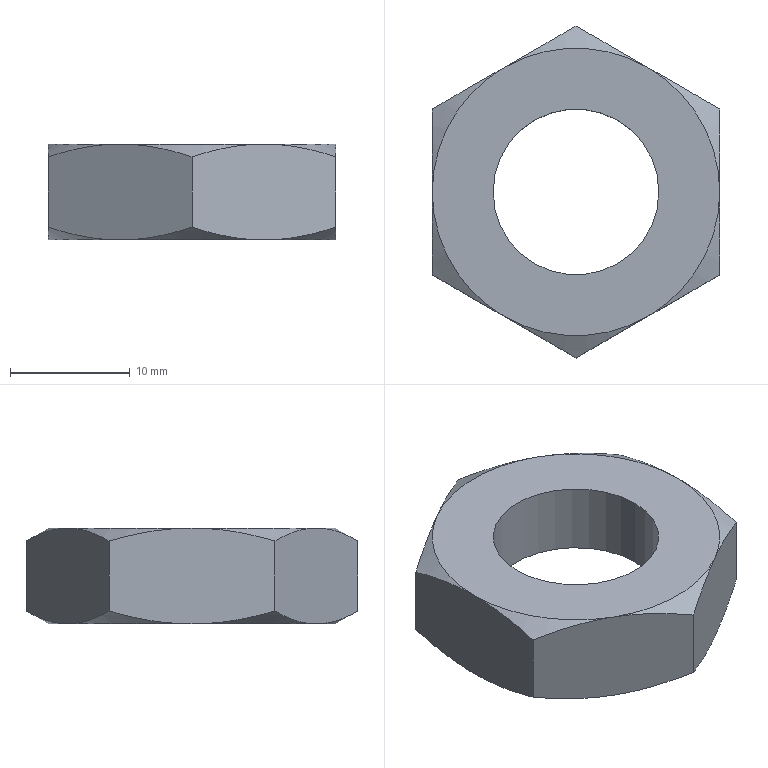Part | STEP file | HXGR200008-06-03-06_M16 | 1 solid | 25 faces | box 24 x 27.713 x 8 mm | volume 2461 mm3 | cone 12 | plane 9 | cylinder 4 | commonest cylinder face diameters 13.835 x2 19.5 x2
STEP:
#1=CARTESIAN_POINT('',(9.75,0.,2.));
#2=VERTEX_POINT('',#1);
#3=CARTESIAN_POINT('',(-9.75,0.,2.));
#4=VERTEX_POINT('',#3);
#5=CARTESIAN_POINT('',(0.,0.,2.));
#6=DIRECTION('',(0.,0.,-1.));
#7=DIRECTION('',(-1.,0.,0.));
#8=AXIS2_PLACEMENT_3D('',#5,#6,#7);
#9=CIRCLE('',#8,9.75);
#10=EDGE_CURVE('',#2,#4,#9,.T.);
#11=ORIENTED_EDGE('',*,*,#10,.F.);
#12=CARTESIAN_POINT('',(9.75,0.,0.));
#13=VERTEX_POINT('',#12);
#14=CARTESIAN_POINT('',(9.75,0.,2.));
#15=DIRECTION('',(0.,0.,-1.));
#16=VECTOR('',#15,1000.);
#17=LINE('',#14,#16);
#18=EDGE_CURVE('',#2,#13,#17,.T.);
#19=ORIENTED_EDGE('',*,*,#18,.T.);
#20=CARTESIAN_POINT('',(-9.75,0.,0.));
#21=VERTEX_POINT('',#20);
#22=CARTESIAN_POINT('',(0.,0.,0.));
#23=DIRECTION('',(0.,0.,-1.));
#24=DIRECTION('',(-1.,0.,0.));
#25=AXIS2_PLACEMENT_3D('',#22,#23,#24);
#26=CIRCLE('',#25,9.75);
#27=EDGE_CURVE('',#13,#21,#26,.T.);
#28=ORIENTED_EDGE('',*,*,#27,.T.);
#29=CARTESIAN_POINT('',(-9.75,0.,2.));
#30=DIRECTION('',(0.,0.,-1.));
#31=VECTOR('',#30,1000.);
#32=LINE('',#29,#31);
#33=EDGE_CURVE('',#4,#21,#32,.T.);
#34=ORIENTED_EDGE('',*,*,#33,.F.);
#35=EDGE_LOOP('',(#11,#19,#28,#34));
#36=FACE_OUTER_BOUND('',#35,.T.);
#37=CARTESIAN_POINT('',(0.,0.,2.));
#38=DIRECTION('',(0.,0.,-1.));
#39=DIRECTION('',(-1.,0.,0.));
#40=AXIS2_PLACEMENT_3D('',#37,#38,#39);
#41=CYLINDRICAL_SURFACE('',#40,9.75);
#42=ADVANCED_FACE('',(#36),#41,.F.);
#43=CARTESIAN_POINT('',(-6.918,0.,8.));
#44=VERTEX_POINT('',#43);
#45=CARTESIAN_POINT('',(6.918,0.,8.));
#46=VERTEX_POINT('',#45);
#47=CARTESIAN_POINT('',(0.,0.,8.));
#48=DIRECTION('',(0.,0.,1.));
#49=DIRECTION('',(1.,0.,0.));
#50=AXIS2_PLACEMENT_3D('',#47,#48,#49);
#51=CIRCLE('',#50,6.918);
#52=EDGE_CURVE('',#44,#46,#51,.T.);
#53=ORIENTED_EDGE('',*,*,#52,.T.);
#54=CARTESIAN_POINT('',(6.918,0.,2.));
#55=VERTEX_POINT('',#54);
#56=CARTESIAN_POINT('',(6.918,0.,8.));
#57=DIRECTION('',(0.,0.,-1.));
#58=VECTOR('',#57,1000.);
#59=LINE('',#56,#58);
#60=EDGE_CURVE('',#46,#55,#59,.T.);
#61=ORIENTED_EDGE('',*,*,#60,.T.);
#62=CARTESIAN_POINT('',(-6.918,0.,2.));
#63=VERTEX_POINT('',#62);
#64=CARTESIAN_POINT('',(0.,0.,2.));
#65=DIRECTION('',(0.,0.,-1.));
#66=DIRECTION('',(-1.,0.,0.));
#67=AXIS2_PLACEMENT_3D('',#64,#65,#66);
#68=CIRCLE('',#67,6.918);
#69=EDGE_CURVE('',#55,#63,#68,.T.);
#70=ORIENTED_EDGE('',*,*,#69,.T.);
#71=CARTESIAN_POINT('',(-6.918,0.,8.));
#72=DIRECTION('',(0.,0.,-1.));
#73=VECTOR('',#72,1000.);
#74=LINE('',#71,#73);
#75=EDGE_CURVE('',#44,#63,#74,.T.);
#76=ORIENTED_EDGE('',*,*,#75,.F.);
#77=EDGE_LOOP('',(#53,#61,#70,#76));
#78=FACE_OUTER_BOUND('',#77,.T.);
#79=CARTESIAN_POINT('',(0.,0.,8.));
#80=DIRECTION('',(0.,0.,-1.));
#81=DIRECTION('',(-1.,0.,0.));
#82=AXIS2_PLACEMENT_3D('',#79,#80,#81);
#83=CYLINDRICAL_SURFACE('',#82,6.918);
#84=ADVANCED_FACE('',(#78),#83,.F.);
#85=ORIENTED_EDGE('',*,*,#60,.F.);
#86=CARTESIAN_POINT('',(0.,0.,8.));
#87=DIRECTION('',(0.,0.,1.));
#88=DIRECTION('',(1.,0.,0.));
#89=AXIS2_PLACEMENT_3D('',#86,#87,#88);
#90=CIRCLE('',#89,6.918);
#91=EDGE_CURVE('',#46,#44,#90,.T.);
#92=ORIENTED_EDGE('',*,*,#91,.T.);
#93=ORIENTED_EDGE('',*,*,#75,.T.);
#94=CARTESIAN_POINT('',(0.,0.,2.));
#95=DIRECTION('',(0.,0.,-1.));
#96=DIRECTION('',(-1.,0.,0.));
#97=AXIS2_PLACEMENT_3D('',#94,#95,#96);
#98=CIRCLE('',#97,6.918);
#99=EDGE_CURVE('',#63,#55,#98,.T.);
#100=ORIENTED_EDGE('',*,*,#99,.T.);
#101=EDGE_LOOP('',(#85,#92,#93,#100));
#102=FACE_OUTER_BOUND('',#101,.T.);
#103=CARTESIAN_POINT('',(0.,0.,8.));
#104=DIRECTION('',(0.,0.,-1.));
#105=DIRECTION('',(-1.,0.,0.));
#106=AXIS2_PLACEMENT_3D('',#103,#104,#105);
#107=CYLINDRICAL_SURFACE('',#106,6.918);
#108=ADVANCED_FACE('',(#102),#107,.F.);
#109=CARTESIAN_POINT('',(12.,6.928,6.928));
#110=VERTEX_POINT('',#109);
#111=CARTESIAN_POINT('',(6.,10.392,8.));
#112=VERTEX_POINT('',#111);
#113=CARTESIAN_POINT('',(12.,6.928,6.928));
#114=CARTESIAN_POINT('',(11.018,7.495,7.255));
#115=CARTESIAN_POINT('',(10.03,8.066,7.525));
#116=CARTESIAN_POINT('',(8.032,9.219,7.898));
#117=CARTESIAN_POINT('',(7.022,9.802,8.));
#118=CARTESIAN_POINT('',(6.,10.392,8.));
#119=B_SPLINE_CURVE_WITH_KNOTS('',3,(#113,#114,#115,#116,#117,#118),.UNSPECIFIED.,.F.,.F.,(4,2,4),(0.000000238,0.003505,0.00701),.UNSPECIFIED.);
#120=EDGE_CURVE('',#110,#112,#119,.T.);
#121=ORIENTED_EDGE('',*,*,#120,.F.);
#122=CARTESIAN_POINT('',(12.,6.928,1.072));
#123=VERTEX_POINT('',#122);
#124=CARTESIAN_POINT('',(12.,6.928,8.));
#125=DIRECTION('',(0.,0.,-1.));
#126=VECTOR('',#125,1000.);
#127=LINE('',#124,#126);
#128=EDGE_CURVE('',#110,#123,#127,.T.);
#129=ORIENTED_EDGE('',*,*,#128,.T.);
#130=CARTESIAN_POINT('',(6.,10.392,0.));
#131=VERTEX_POINT('',#130);
#132=CARTESIAN_POINT('',(6.,10.392,0.));
#133=CARTESIAN_POINT('',(6.509,10.098,0.));
#134=CARTESIAN_POINT('',(7.021,9.803,0.02533));
#135=CARTESIAN_POINT('',(8.033,9.219,0.1234));
#136=CARTESIAN_POINT('',(8.535,8.929,0.196));
#137=CARTESIAN_POINT('',(10.034,8.063,0.476));
#138=CARTESIAN_POINT('',(11.021,7.493,0.7454));
#139=CARTESIAN_POINT('',(12.,6.928,1.072));
#140=B_SPLINE_CURVE_WITH_KNOTS('',3,(#132,#133,#134,#135,#136,#137,#138,#139),.UNSPECIFIED.,.F.,.F.,(4,2,2,4),(0.00701,0.008756,0.0105,0.01399),.UNSPECIFIED.);
#141=EDGE_CURVE('',#131,#123,#140,.T.);
#142=ORIENTED_EDGE('',*,*,#141,.F.);
#143=CARTESIAN_POINT('',(0.,13.856,1.072));
#144=VERTEX_POINT('',#143);
#145=CARTESIAN_POINT('',(0.,13.856,1.072));
#146=CARTESIAN_POINT('',(0.9815,13.29,0.7446));
#147=CARTESIAN_POINT('',(1.97,12.719,0.4751));
#148=CARTESIAN_POINT('',(3.968,11.565,0.1021));
#149=CARTESIAN_POINT('',(4.978,10.982,0.));
#150=CARTESIAN_POINT('',(6.,10.392,0.));
#151=B_SPLINE_CURVE_WITH_KNOTS('',3,(#145,#146,#147,#148,#149,#150),.UNSPECIFIED.,.F.,.F.,(4,2,4),(0.000000238,0.003505,0.00701),.UNSPECIFIED.);
#152=EDGE_CURVE('',#144,#131,#151,.T.);
#153=ORIENTED_EDGE('',*,*,#152,.F.);
#154=CARTESIAN_POINT('',(0.,13.856,6.928));
#155=VERTEX_POINT('',#154);
#156=CARTESIAN_POINT('',(0.,13.856,8.));
#157=DIRECTION('',(0.,0.,-1.));
#158=VECTOR('',#157,1000.);
#159=LINE('',#156,#158);
#160=EDGE_CURVE('',#155,#144,#159,.T.);
#161=ORIENTED_EDGE('',*,*,#160,.F.);
#162=CARTESIAN_POINT('',(6.,10.392,8.));
#163=CARTESIAN_POINT('',(5.491,10.686,8.));
#164=CARTESIAN_POINT('',(4.979,10.982,7.975));
#165=CARTESIAN_POINT('',(3.967,11.566,7.877));
#166=CARTESIAN_POINT('',(3.465,11.856,7.804));
#167=CARTESIAN_POINT('',(1.966,12.721,7.524));
#168=CARTESIAN_POINT('',(0.9791,13.291,7.255));
#169=CARTESIAN_POINT('',(0.,13.856,6.928));
#170=B_SPLINE_CURVE_WITH_KNOTS('',3,(#162,#163,#164,#165,#166,#167,#168,#169),.UNSPECIFIED.,.F.,.F.,(4,2,2,4),(0.00701,0.008756,0.0105,0.01399),.UNSPECIFIED.);
#171=EDGE_CURVE('',#112,#155,#170,.T.);
#172=ORIENTED_EDGE('',*,*,#171,.F.);
#173=EDGE_LOOP('',(#121,#129,#142,#153,#161,#172));
#174=FACE_OUTER_BOUND('',#173,.T.);
#175=CARTESIAN_POINT('',(12.,6.928,8.));
#176=DIRECTION('',(-0.5,-0.866,0.));
#177=DIRECTION('',(0.866,-0.5,0.));
#178=AXIS2_PLACEMENT_3D('',#175,#176,#177);
#179=PLANE('',#178);
#180=ADVANCED_FACE('',(#174),#179,.F.);
#181=CARTESIAN_POINT('',(-6.,10.392,8.));
#182=VERTEX_POINT('',#181);
#183=CARTESIAN_POINT('',(0.,13.856,6.928));
#184=CARTESIAN_POINT('',(-0.9815,13.29,7.255));
#185=CARTESIAN_POINT('',(-1.97,12.719,7.525));
#186=CARTESIAN_POINT('',(-3.968,11.565,7.898));
#187=CARTESIAN_POINT('',(-4.978,10.982,8.));
#188=CARTESIAN_POINT('',(-6.,10.392,8.));
#189=B_SPLINE_CURVE_WITH_KNOTS('',3,(#183,#184,#185,#186,#187,#188),.UNSPECIFIED.,.F.,.F.,(4,2,4),(0.000000238,0.003505,0.00701),.UNSPECIFIED.);
#190=EDGE_CURVE('',#155,#182,#189,.T.);
#191=ORIENTED_EDGE('',*,*,#190,.F.);
#192=ORIENTED_EDGE('',*,*,#160,.T.);
#193=CARTESIAN_POINT('',(-6.,10.392,0.));
#194=VERTEX_POINT('',#193);
#195=CARTESIAN_POINT('',(-6.,10.392,0.));
#196=CARTESIAN_POINT('',(-5.491,10.686,0.));
#197=CARTESIAN_POINT('',(-4.979,10.982,0.02533));
#198=CARTESIAN_POINT('',(-3.967,11.566,0.1234));
#199=CARTESIAN_POINT('',(-3.465,11.856,0.196));
#200=CARTESIAN_POINT('',(-1.966,12.721,0.476));
#201=CARTESIAN_POINT('',(-0.9791,13.291,0.7454));
#202=CARTESIAN_POINT('',(0.,13.856,1.072));
#203=B_SPLINE_CURVE_WITH_KNOTS('',3,(#195,#196,#197,#198,#199,#200,#201,#202),.UNSPECIFIED.,.F.,.F.,(4,2,2,4),(0.00701,0.008756,0.0105,0.01399),.UNSPECIFIED.);
#204=EDGE_CURVE('',#194,#144,#203,.T.);
#205=ORIENTED_EDGE('',*,*,#204,.F.);
#206=CARTESIAN_POINT('',(-12.,6.928,1.072));
#207=VERTEX_POINT('',#206);
#208=CARTESIAN_POINT('',(-12.,6.928,1.072));
#209=CARTESIAN_POINT('',(-11.018,7.495,0.7446));
#210=CARTESIAN_POINT('',(-10.03,8.066,0.4751));
#211=CARTESIAN_POINT('',(-8.032,9.219,0.1021));
#212=CARTESIAN_POINT('',(-7.022,9.802,0.));
#213=CARTESIAN_POINT('',(-6.,10.392,0.));
#214=B_SPLINE_CURVE_WITH_KNOTS('',3,(#208,#209,#210,#211,#212,#213),.UNSPECIFIED.,.F.,.F.,(4,2,4),(0.000000238,0.003505,0.00701),.UNSPECIFIED.);
#215=EDGE_CURVE('',#207,#194,#214,.T.);
#216=ORIENTED_EDGE('',*,*,#215,.F.);
#217=CARTESIAN_POINT('',(-12.,6.928,6.928));
#218=VERTEX_POINT('',#217);
#219=CARTESIAN_POINT('',(-12.,6.928,8.));
#220=DIRECTION('',(0.,0.,-1.));
#221=VECTOR('',#220,1000.);
#222=LINE('',#219,#221);
#223=EDGE_CURVE('',#218,#207,#222,.T.);
#224=ORIENTED_EDGE('',*,*,#223,.F.);
#225=CARTESIAN_POINT('',(-6.,10.392,8.));
#226=CARTESIAN_POINT('',(-6.509,10.098,8.));
#227=CARTESIAN_POINT('',(-7.021,9.803,7.975));
#228=CARTESIAN_POINT('',(-8.033,9.219,7.877));
#229=CARTESIAN_POINT('',(-8.535,8.929,7.804));
#230=CARTESIAN_POINT('',(-10.034,8.063,7.524));
#231=CARTESIAN_POINT('',(-11.021,7.493,7.255));
#232=CARTESIAN_POINT('',(-12.,6.928,6.928));
#233=B_SPLINE_CURVE_WITH_KNOTS('',3,(#225,#226,#227,#228,#229,#230,#231,#232),.UNSPECIFIED.,.F.,.F.,(4,2,2,4),(0.00701,0.008756,0.0105,0.01399),.UNSPECIFIED.);
#234=EDGE_CURVE('',#182,#218,#233,.T.);
#235=ORIENTED_EDGE('',*,*,#234,.F.);
#236=EDGE_LOOP('',(#191,#192,#205,#216,#224,#235));
#237=FACE_OUTER_BOUND('',#236,.T.);
#238=CARTESIAN_POINT('',(0.,13.856,8.));
#239=DIRECTION('',(0.5,-0.866,0.));
#240=DIRECTION('',(0.866,0.5,0.));
#241=AXIS2_PLACEMENT_3D('',#238,#239,#240);
#242=PLANE('',#241);
#243=ADVANCED_FACE('',(#237),#242,.F.);
#244=CARTESIAN_POINT('',(-12.,0.,8.));
#245=VERTEX_POINT('',#244);
#246=CARTESIAN_POINT('',(-12.,6.928,6.928));
#247=CARTESIAN_POINT('',(-12.,5.808,7.252));
#248=CARTESIAN_POINT('',(-12.,4.673,7.521));
#249=CARTESIAN_POINT('',(-12.,2.939,7.802));
#250=CARTESIAN_POINT('',(-12.,2.355,7.876));
#251=CARTESIAN_POINT('',(-12.,1.176,7.975));
#252=CARTESIAN_POINT('',(-12.,0.5865,8.));
#253=CARTESIAN_POINT('',(-12.,0.,8.));
#254=B_SPLINE_CURVE_WITH_KNOTS('',3,(#246,#247,#248,#249,#250,#251,#252,#253),.UNSPECIFIED.,.F.,.F.,(4,2,2,4),(0.03616,0.03967,0.04143,0.04318),.UNSPECIFIED.);
#255=EDGE_CURVE('',#218,#245,#254,.T.);
#256=ORIENTED_EDGE('',*,*,#255,.F.);
#257=ORIENTED_EDGE('',*,*,#223,.T.);
#258=CARTESIAN_POINT('',(-12.,0.,0.));
#259=VERTEX_POINT('',#258);
#260=CARTESIAN_POINT('',(-12.,0.,0.));
#261=CARTESIAN_POINT('',(-12.,0.5865,0.));
#262=CARTESIAN_POINT('',(-12.,1.176,0.02506));
#263=CARTESIAN_POINT('',(-12.,2.355,0.1242));
#264=CARTESIAN_POINT('',(-12.,2.939,0.1976));
#265=CARTESIAN_POINT('',(-12.,4.673,0.4791));
#266=CARTESIAN_POINT('',(-12.,5.808,0.7483));
#267=CARTESIAN_POINT('',(-12.,6.928,1.072));
#268=B_SPLINE_CURVE_WITH_KNOTS('',3,(#260,#261,#262,#263,#264,#265,#266,#267),.UNSPECIFIED.,.F.,.F.,(4,2,2,4),(0.01983,0.02158,0.02334,0.02685),.UNSPECIFIED.);
#269=EDGE_CURVE('',#259,#207,#268,.T.);
#270=ORIENTED_EDGE('',*,*,#269,.F.);
#271=CARTESIAN_POINT('',(-12.,-6.928,1.072));
#272=VERTEX_POINT('',#271);
#273=CARTESIAN_POINT('',(-12.,-6.928,1.072));
#274=CARTESIAN_POINT('',(-12.,-5.8,0.7461));
#275=CARTESIAN_POINT('',(-12.,-4.647,0.4736));
#276=CARTESIAN_POINT('',(-12.,-2.335,0.1008));
#277=CARTESIAN_POINT('',(-12.,-1.172,0.));
#278=CARTESIAN_POINT('',(-12.,0.,0.));
#279=B_SPLINE_CURVE_WITH_KNOTS('',3,(#273,#274,#275,#276,#277,#278),.UNSPECIFIED.,.F.,.F.,(4,2,4),(0.01282,0.01632,0.01983),.UNSPECIFIED.);
#280=EDGE_CURVE('',#272,#259,#279,.T.);
#281=ORIENTED_EDGE('',*,*,#280,.F.);
#282=CARTESIAN_POINT('',(-12.,-6.928,6.928));
#283=VERTEX_POINT('',#282);
#284=CARTESIAN_POINT('',(-12.,-6.928,8.));
#285=DIRECTION('',(0.,0.,-1.));
#286=VECTOR('',#285,1000.);
#287=LINE('',#284,#286);
#288=EDGE_CURVE('',#283,#272,#287,.T.);
#289=ORIENTED_EDGE('',*,*,#288,.F.);
#290=CARTESIAN_POINT('',(-12.,0.,8.));
#291=CARTESIAN_POINT('',(-12.,-1.172,8.));
#292=CARTESIAN_POINT('',(-12.,-2.335,7.899));
#293=CARTESIAN_POINT('',(-12.,-4.647,7.526));
#294=CARTESIAN_POINT('',(-12.,-5.8,7.254));
#295=CARTESIAN_POINT('',(-12.,-6.928,6.928));
#296=B_SPLINE_CURVE_WITH_KNOTS('',3,(#290,#291,#292,#293,#294,#295),.UNSPECIFIED.,.F.,.F.,(4,2,4),(0.04318,0.04669,0.05019),.UNSPECIFIED.);
#297=EDGE_CURVE('',#245,#283,#296,.T.);
#298=ORIENTED_EDGE('',*,*,#297,.F.);
#299=EDGE_LOOP('',(#256,#257,#270,#281,#289,#298));
#300=FACE_OUTER_BOUND('',#299,.T.);
#301=CARTESIAN_POINT('',(-12.,6.928,8.));
#302=DIRECTION('',(1.,0.,0.));
#303=DIRECTION('',(0.,1.,0.));
#304=AXIS2_PLACEMENT_3D('',#301,#302,#303);
#305=PLANE('',#304);
#306=ADVANCED_FACE('',(#300),#305,.F.);
#307=CARTESIAN_POINT('',(-6.,-10.392,8.));
#308=VERTEX_POINT('',#307);
#309=CARTESIAN_POINT('',(-12.,-6.928,6.928));
#310=CARTESIAN_POINT('',(-11.018,-7.495,7.255));
#311=CARTESIAN_POINT('',(-10.03,-8.066,7.525));
#312=CARTESIAN_POINT('',(-8.032,-9.219,7.898));
#313=CARTESIAN_POINT('',(-7.022,-9.802,8.));
#314=CARTESIAN_POINT('',(-6.,-10.392,8.));
#315=B_SPLINE_CURVE_WITH_KNOTS('',3,(#309,#310,#311,#312,#313,#314),.UNSPECIFIED.,.F.,.F.,(4,2,4),(0.000000238,0.003505,0.00701),.UNSPECIFIED.);
#316=EDGE_CURVE('',#283,#308,#315,.T.);
#317=ORIENTED_EDGE('',*,*,#316,.F.);
#318=ORIENTED_EDGE('',*,*,#288,.T.);
#319=CARTESIAN_POINT('',(-6.,-10.392,0.));
#320=VERTEX_POINT('',#319);
#321=CARTESIAN_POINT('',(-6.,-10.392,0.));
#322=CARTESIAN_POINT('',(-6.509,-10.098,0.));
#323=CARTESIAN_POINT('',(-7.021,-9.803,0.02533));
#324=CARTESIAN_POINT('',(-8.033,-9.219,0.1234));
#325=CARTESIAN_POINT('',(-8.535,-8.929,0.196));
#326=CARTESIAN_POINT('',(-10.034,-8.063,0.476));
#327=CARTESIAN_POINT('',(-11.021,-7.493,0.7454));
#328=CARTESIAN_POINT('',(-12.,-6.928,1.072));
#329=B_SPLINE_CURVE_WITH_KNOTS('',3,(#321,#322,#323,#324,#325,#326,#327,#328),.UNSPECIFIED.,.F.,.F.,(4,2,2,4),(0.00701,0.008756,0.0105,0.01399),.UNSPECIFIED.);
#330=EDGE_CURVE('',#320,#272,#329,.T.);
#331=ORIENTED_EDGE('',*,*,#330,.F.);
#332=CARTESIAN_POINT('',(0.,-13.856,1.072));
#333=VERTEX_POINT('',#332);
#334=CARTESIAN_POINT('',(0.,-13.856,1.072));
#335=CARTESIAN_POINT('',(-0.9815,-13.29,0.7446));
#336=CARTESIAN_POINT('',(-1.97,-12.719,0.4751));
#337=CARTESIAN_POINT('',(-3.968,-11.565,0.1021));
#338=CARTESIAN_POINT('',(-4.978,-10.982,0.));
#339=CARTESIAN_POINT('',(-6.,-10.392,0.));
#340=B_SPLINE_CURVE_WITH_KNOTS('',3,(#334,#335,#336,#337,#338,#339),.UNSPECIFIED.,.F.,.F.,(4,2,4),(0.000000238,0.003505,0.00701),.UNSPECIFIED.);
#341=EDGE_CURVE('',#333,#320,#340,.T.);
#342=ORIENTED_EDGE('',*,*,#341,.F.);
#343=CARTESIAN_POINT('',(0.,-13.856,6.928));
#344=VERTEX_POINT('',#343);
#345=CARTESIAN_POINT('',(0.,-13.856,8.));
#346=DIRECTION('',(0.,0.,-1.));
#347=VECTOR('',#346,1000.);
#348=LINE('',#345,#347);
#349=EDGE_CURVE('',#344,#333,#348,.T.);
#350=ORIENTED_EDGE('',*,*,#349,.F.);
#351=CARTESIAN_POINT('',(-6.,-10.392,8.));
#352=CARTESIAN_POINT('',(-5.491,-10.686,8.));
#353=CARTESIAN_POINT('',(-4.979,-10.982,7.975));
#354=CARTESIAN_POINT('',(-3.967,-11.566,7.877));
#355=CARTESIAN_POINT('',(-3.465,-11.856,7.804));
#356=CARTESIAN_POINT('',(-1.966,-12.721,7.524));
#357=CARTESIAN_POINT('',(-0.9791,-13.291,7.255));
#358=CARTESIAN_POINT('',(0.,-13.856,6.928));
#359=B_SPLINE_CURVE_WITH_KNOTS('',3,(#351,#352,#353,#354,#355,#356,#357,#358),.UNSPECIFIED.,.F.,.F.,(4,2,2,4),(0.00701,0.008756,0.0105,0.01399),.UNSPECIFIED.);
#360=EDGE_CURVE('',#308,#344,#359,.T.);
#361=ORIENTED_EDGE('',*,*,#360,.F.);
#362=EDGE_LOOP('',(#317,#318,#331,#342,#350,#361));
#363=FACE_OUTER_BOUND('',#362,.T.);
#364=CARTESIAN_POINT('',(-12.,-6.928,8.));
#365=DIRECTION('',(0.5,0.866,0.));
#366=DIRECTION('',(-0.866,0.5,0.));
#367=AXIS2_PLACEMENT_3D('',#364,#365,#366);
#368=PLANE('',#367);
#369=ADVANCED_FACE('',(#363),#368,.F.);
#370=CARTESIAN_POINT('',(6.,-10.392,8.));
#371=VERTEX_POINT('',#370);
#372=CARTESIAN_POINT('',(0.,-13.856,6.928));
#373=CARTESIAN_POINT('',(0.9815,-13.29,7.255));
#374=CARTESIAN_POINT('',(1.97,-12.719,7.525));
#375=CARTESIAN_POINT('',(3.968,-11.565,7.898));
#376=CARTESIAN_POINT('',(4.978,-10.982,8.));
#377=CARTESIAN_POINT('',(6.,-10.392,8.));
#378=B_SPLINE_CURVE_WITH_KNOTS('',3,(#372,#373,#374,#375,#376,#377),.UNSPECIFIED.,.F.,.F.,(4,2,4),(0.000000238,0.003505,0.00701),.UNSPECIFIED.);
#379=EDGE_CURVE('',#344,#371,#378,.T.);
#380=ORIENTED_EDGE('',*,*,#379,.F.);
#381=ORIENTED_EDGE('',*,*,#349,.T.);
#382=CARTESIAN_POINT('',(6.,-10.392,0.));
#383=VERTEX_POINT('',#382);
#384=CARTESIAN_POINT('',(6.,-10.392,0.));
#385=CARTESIAN_POINT('',(5.491,-10.686,0.));
#386=CARTESIAN_POINT('',(4.979,-10.982,0.02533));
#387=CARTESIAN_POINT('',(3.967,-11.566,0.1234));
#388=CARTESIAN_POINT('',(3.465,-11.856,0.196));
#389=CARTESIAN_POINT('',(1.966,-12.721,0.476));
#390=CARTESIAN_POINT('',(0.9791,-13.291,0.7454));
#391=CARTESIAN_POINT('',(0.,-13.856,1.072));
#392=B_SPLINE_CURVE_WITH_KNOTS('',3,(#384,#385,#386,#387,#388,#389,#390,#391),.UNSPECIFIED.,.F.,.F.,(4,2,2,4),(0.00701,0.008756,0.0105,0.01399),.UNSPECIFIED.);
#393=EDGE_CURVE('',#383,#333,#392,.T.);
#394=ORIENTED_EDGE('',*,*,#393,.F.);
#395=CARTESIAN_POINT('',(12.,-6.928,1.072));
#396=VERTEX_POINT('',#395);
#397=CARTESIAN_POINT('',(12.,-6.928,1.072));
#398=CARTESIAN_POINT('',(11.018,-7.495,0.7446));
#399=CARTESIAN_POINT('',(10.03,-8.066,0.4751));
#400=CARTESIAN_POINT('',(8.032,-9.219,0.1021));
#401=CARTESIAN_POINT('',(7.022,-9.802,0.));
#402=CARTESIAN_POINT('',(6.,-10.392,0.));
#403=B_SPLINE_CURVE_WITH_KNOTS('',3,(#397,#398,#399,#400,#401,#402),.UNSPECIFIED.,.F.,.F.,(4,2,4),(0.000000238,0.003505,0.00701),.UNSPECIFIED.);
#404=EDGE_CURVE('',#396,#383,#403,.T.);
#405=ORIENTED_EDGE('',*,*,#404,.F.);
#406=CARTESIAN_POINT('',(12.,-6.928,6.928));
#407=VERTEX_POINT('',#406);
#408=CARTESIAN_POINT('',(12.,-6.928,8.));
#409=DIRECTION('',(0.,0.,-1.));
#410=VECTOR('',#409,1000.);
#411=LINE('',#408,#410);
#412=EDGE_CURVE('',#407,#396,#411,.T.);
#413=ORIENTED_EDGE('',*,*,#412,.F.);
#414=CARTESIAN_POINT('',(6.,-10.392,8.));
#415=CARTESIAN_POINT('',(6.509,-10.098,8.));
#416=CARTESIAN_POINT('',(7.021,-9.803,7.975));
#417=CARTESIAN_POINT('',(8.033,-9.219,7.877));
#418=CARTESIAN_POINT('',(8.535,-8.929,7.804));
#419=CARTESIAN_POINT('',(10.034,-8.063,7.524));
#420=CARTESIAN_POINT('',(11.021,-7.493,7.255));
#421=CARTESIAN_POINT('',(12.,-6.928,6.928));
#422=B_SPLINE_CURVE_WITH_KNOTS('',3,(#414,#415,#416,#417,#418,#419,#420,#421),.UNSPECIFIED.,.F.,.F.,(4,2,2,4),(0.00701,0.008756,0.0105,0.01399),.UNSPECIFIED.);
#423=EDGE_CURVE('',#371,#407,#422,.T.);
#424=ORIENTED_EDGE('',*,*,#423,.F.);
#425=EDGE_LOOP('',(#380,#381,#394,#405,#413,#424));
#426=FACE_OUTER_BOUND('',#425,.T.);
#427=CARTESIAN_POINT('',(0.,-13.856,8.));
#428=DIRECTION('',(-0.5,0.866,0.));
#429=DIRECTION('',(-0.866,-0.5,0.));
#430=AXIS2_PLACEMENT_3D('',#427,#428,#429);
#431=PLANE('',#430);
#432=ADVANCED_FACE('',(#426),#431,.F.);
#433=CARTESIAN_POINT('',(12.,0.,8.));
#434=VERTEX_POINT('',#433);
#435=CARTESIAN_POINT('',(12.,-6.928,6.928));
#436=CARTESIAN_POINT('',(12.,-5.8,7.254));
#437=CARTESIAN_POINT('',(12.,-4.647,7.526));
#438=CARTESIAN_POINT('',(12.,-2.335,7.899));
#439=CARTESIAN_POINT('',(12.,-1.172,8.));
#440=CARTESIAN_POINT('',(12.,0.,8.));
#441=B_SPLINE_CURVE_WITH_KNOTS('',3,(#435,#436,#437,#438,#439,#440),.UNSPECIFIED.,.F.,.F.,(4,2,4),(0.01282,0.01632,0.01983),.UNSPECIFIED.);
#442=EDGE_CURVE('',#407,#434,#441,.T.);
#443=ORIENTED_EDGE('',*,*,#442,.F.);
#444=ORIENTED_EDGE('',*,*,#412,.T.);
#445=CARTESIAN_POINT('',(12.,0.,0.));
#446=VERTEX_POINT('',#445);
#447=CARTESIAN_POINT('',(12.,0.,0.));
#448=CARTESIAN_POINT('',(12.,-1.172,0.));
#449=CARTESIAN_POINT('',(12.,-2.335,0.1008));
#450=CARTESIAN_POINT('',(12.,-4.647,0.4736));
#451=CARTESIAN_POINT('',(12.,-5.8,0.7461));
#452=CARTESIAN_POINT('',(12.,-6.928,1.072));
#453=B_SPLINE_CURVE_WITH_KNOTS('',3,(#447,#448,#449,#450,#451,#452),.UNSPECIFIED.,.F.,.F.,(4,2,4),(0.04318,0.04669,0.05019),.UNSPECIFIED.);
#454=EDGE_CURVE('',#446,#396,#453,.T.);
#455=ORIENTED_EDGE('',*,*,#454,.F.);
#456=CARTESIAN_POINT('',(12.,6.928,1.072));
#457=CARTESIAN_POINT('',(12.,5.808,0.7483));
#458=CARTESIAN_POINT('',(12.,4.673,0.4791));
#459=CARTESIAN_POINT('',(12.,2.939,0.1976));
#460=CARTESIAN_POINT('',(12.,2.355,0.1242));
#461=CARTESIAN_POINT('',(12.,1.176,0.02506));
#462=CARTESIAN_POINT('',(12.,0.5865,0.));
#463=CARTESIAN_POINT('',(12.,0.,0.));
#464=B_SPLINE_CURVE_WITH_KNOTS('',3,(#456,#457,#458,#459,#460,#461,#462,#463),.UNSPECIFIED.,.F.,.F.,(4,2,2,4),(0.03616,0.03967,0.04143,0.04318),.UNSPECIFIED.);
#465=EDGE_CURVE('',#123,#446,#464,.T.);
#466=ORIENTED_EDGE('',*,*,#465,.F.);
#467=ORIENTED_EDGE('',*,*,#128,.F.);
#468=CARTESIAN_POINT('',(12.,0.,8.));
#469=CARTESIAN_POINT('',(12.,0.5865,8.));
#470=CARTESIAN_POINT('',(12.,1.176,7.975));
#471=CARTESIAN_POINT('',(12.,2.355,7.876));
#472=CARTESIAN_POINT('',(12.,2.939,7.802));
#473=CARTESIAN_POINT('',(12.,4.673,7.521));
#474=CARTESIAN_POINT('',(12.,5.808,7.252));
#475=CARTESIAN_POINT('',(12.,6.928,6.928));
#476=B_SPLINE_CURVE_WITH_KNOTS('',3,(#468,#469,#470,#471,#472,#473,#474,#475),.UNSPECIFIED.,.F.,.F.,(4,2,2,4),(0.01983,0.02158,0.02334,0.02685),.UNSPECIFIED.);
#477=EDGE_CURVE('',#434,#110,#476,.T.);
#478=ORIENTED_EDGE('',*,*,#477,.F.);
#479=EDGE_LOOP('',(#443,#444,#455,#466,#467,#478));
#480=FACE_OUTER_BOUND('',#479,.T.);
#481=CARTESIAN_POINT('',(12.,-6.928,8.));
#482=DIRECTION('',(-1.,0.,0.));
#483=DIRECTION('',(0.,-1.,0.));
#484=AXIS2_PLACEMENT_3D('',#481,#482,#483);
#485=PLANE('',#484);
#486=ADVANCED_FACE('',(#480),#485,.F.);
#487=ORIENTED_EDGE('',*,*,#52,.F.);
#488=ORIENTED_EDGE('',*,*,#91,.F.);
#489=EDGE_LOOP('',(#487,#488));
#490=FACE_BOUND('',#489,.T.);
#491=CARTESIAN_POINT('',(0.,0.,8.));
#492=DIRECTION('',(0.,0.,-1.));
#493=DIRECTION('',(-1.,0.,0.));
#494=AXIS2_PLACEMENT_3D('',#491,#492,#493);
#495=CIRCLE('',#494,12.);
#496=EDGE_CURVE('',#245,#182,#495,.T.);
#497=ORIENTED_EDGE('',*,*,#496,.F.);
#498=CARTESIAN_POINT('',(0.,0.,8.));
#499=DIRECTION('',(0.,0.,-1.));
#500=DIRECTION('',(-1.,0.,0.));
#501=AXIS2_PLACEMENT_3D('',#498,#499,#500);
#502=CIRCLE('',#501,12.);
#503=EDGE_CURVE('',#308,#245,#502,.T.);
#504=ORIENTED_EDGE('',*,*,#503,.F.);
#505=CARTESIAN_POINT('',(0.,0.,8.));
#506=DIRECTION('',(0.,0.,-1.));
#507=DIRECTION('',(-1.,0.,0.));
#508=AXIS2_PLACEMENT_3D('',#505,#506,#507);
#509=CIRCLE('',#508,12.);
#510=EDGE_CURVE('',#371,#308,#509,.T.);
#511=ORIENTED_EDGE('',*,*,#510,.F.);
#512=CARTESIAN_POINT('',(0.,0.,8.));
#513=DIRECTION('',(0.,0.,-1.));
#514=DIRECTION('',(-1.,0.,0.));
#515=AXIS2_PLACEMENT_3D('',#512,#513,#514);
#516=CIRCLE('',#515,12.);
#517=EDGE_CURVE('',#434,#371,#516,.T.);
#518=ORIENTED_EDGE('',*,*,#517,.F.);
#519=CARTESIAN_POINT('',(0.,0.,8.));
#520=DIRECTION('',(0.,0.,1.));
#521=DIRECTION('',(1.,0.,0.));
#522=AXIS2_PLACEMENT_3D('',#519,#520,#521);
#523=CIRCLE('',#522,12.);
#524=EDGE_CURVE('',#434,#112,#523,.T.);
#525=ORIENTED_EDGE('',*,*,#524,.T.);
#526=CARTESIAN_POINT('',(0.,0.,8.));
#527=DIRECTION('',(0.,0.,-1.));
#528=DIRECTION('',(-1.,0.,0.));
#529=AXIS2_PLACEMENT_3D('',#526,#527,#528);
#530=CIRCLE('',#529,12.);
#531=EDGE_CURVE('',#182,#112,#530,.T.);
#532=ORIENTED_EDGE('',*,*,#531,.F.);
#533=EDGE_LOOP('',(#497,#504,#511,#518,#525,#532));
#534=FACE_OUTER_BOUND('',#533,.T.);
#535=CARTESIAN_POINT('',(12.,6.928,8.));
#536=DIRECTION('',(0.,0.,-1.));
#537=DIRECTION('',(-1.,0.,0.));
#538=AXIS2_PLACEMENT_3D('',#535,#536,#537);
#539=PLANE('',#538);
#540=ADVANCED_FACE('',(#490,#534),#539,.F.);
#541=CARTESIAN_POINT('',(0.,0.,0.));
#542=DIRECTION('',(0.,0.,-1.));
#543=DIRECTION('',(-1.,0.,0.));
#544=AXIS2_PLACEMENT_3D('',#541,#542,#543);
#545=CIRCLE('',#544,9.75);
#546=EDGE_CURVE('',#21,#13,#545,.T.);
#547=ORIENTED_EDGE('',*,*,#546,.F.);
#548=ORIENTED_EDGE('',*,*,#27,.F.);
#549=EDGE_LOOP('',(#547,#548));
#550=FACE_BOUND('',#549,.T.);
#551=CARTESIAN_POINT('',(0.,0.,0.));
#552=DIRECTION('',(0.,0.,-1.));
#553=DIRECTION('',(-1.,0.,0.));
#554=AXIS2_PLACEMENT_3D('',#551,#552,#553);
#555=CIRCLE('',#554,12.);
#556=EDGE_CURVE('',#320,#259,#555,.T.);
#557=ORIENTED_EDGE('',*,*,#556,.T.);
#558=CARTESIAN_POINT('',(0.,0.,0.));
#559=DIRECTION('',(0.,0.,-1.));
#560=DIRECTION('',(-1.,0.,0.));
#561=AXIS2_PLACEMENT_3D('',#558,#559,#560);
#562=CIRCLE('',#561,12.);
#563=EDGE_CURVE('',#259,#194,#562,.T.);
#564=ORIENTED_EDGE('',*,*,#563,.T.);
#565=CARTESIAN_POINT('',(0.,0.,0.));
#566=DIRECTION('',(0.,0.,-1.));
#567=DIRECTION('',(-1.,0.,0.));
#568=AXIS2_PLACEMENT_3D('',#565,#566,#567);
#569=CIRCLE('',#568,12.);
#570=EDGE_CURVE('',#194,#131,#569,.T.);
#571=ORIENTED_EDGE('',*,*,#570,.T.);
#572=CARTESIAN_POINT('',(0.,0.,0.));
#573=DIRECTION('',(0.,0.,-1.));
#574=DIRECTION('',(-1.,0.,0.));
#575=AXIS2_PLACEMENT_3D('',#572,#573,#574);
#576=CIRCLE('',#575,12.);
#577=EDGE_CURVE('',#131,#446,#576,.T.);
#578=ORIENTED_EDGE('',*,*,#577,.T.);
#579=CARTESIAN_POINT('',(0.,0.,0.));
#580=DIRECTION('',(0.,0.,-1.));
#581=DIRECTION('',(-1.,0.,0.));
#582=AXIS2_PLACEMENT_3D('',#579,#580,#581);
#583=CIRCLE('',#582,12.);
#584=EDGE_CURVE('',#446,#383,#583,.T.);
#585=ORIENTED_EDGE('',*,*,#584,.T.);
#586=CARTESIAN_POINT('',(0.,0.,0.));
#587=DIRECTION('',(0.,0.,-1.));
#588=DIRECTION('',(-1.,0.,0.));
#589=AXIS2_PLACEMENT_3D('',#586,#587,#588);
#590=CIRCLE('',#589,12.);
#591=EDGE_CURVE('',#383,#320,#590,.T.);
#592=ORIENTED_EDGE('',*,*,#591,.T.);
#593=EDGE_LOOP('',(#557,#564,#571,#578,#585,#592));
#594=FACE_OUTER_BOUND('',#593,.T.);
#595=CARTESIAN_POINT('',(12.,6.928,0.));
#596=DIRECTION('',(0.,0.,-1.));
#597=DIRECTION('',(-1.,0.,0.));
#598=AXIS2_PLACEMENT_3D('',#595,#596,#597);
#599=PLANE('',#598);
#600=ADVANCED_FACE('',(#550,#594),#599,.T.);
#601=ORIENTED_EDGE('',*,*,#404,.T.);
#602=ORIENTED_EDGE('',*,*,#584,.F.);
#603=ORIENTED_EDGE('',*,*,#454,.T.);
#604=EDGE_LOOP('',(#601,#602,#603));
#605=FACE_OUTER_BOUND('',#604,.T.);
#606=CARTESIAN_POINT('',(0.,0.,0.));
#607=DIRECTION('',(0.,0.,1.));
#608=DIRECTION('',(-1.,0.,0.));
#609=AXIS2_PLACEMENT_3D('',#606,#607,#608);
#610=CONICAL_SURFACE('',#609,12.,1.047);
#611=ADVANCED_FACE('',(#605),#610,.T.);
#612=ORIENTED_EDGE('',*,*,#141,.T.);
#613=ORIENTED_EDGE('',*,*,#465,.T.);
#614=ORIENTED_EDGE('',*,*,#577,.F.);
#615=EDGE_LOOP('',(#612,#613,#614));
#616=FACE_OUTER_BOUND('',#615,.T.);
#617=CARTESIAN_POINT('',(0.,0.,0.));
#618=DIRECTION('',(0.,0.,1.));
#619=DIRECTION('',(-1.,0.,0.));
#620=AXIS2_PLACEMENT_3D('',#617,#618,#619);
#621=CONICAL_SURFACE('',#620,12.,1.047);
#622=ADVANCED_FACE('',(#616),#621,.T.);
#623=ORIENTED_EDGE('',*,*,#341,.T.);
#624=ORIENTED_EDGE('',*,*,#591,.F.);
#625=ORIENTED_EDGE('',*,*,#393,.T.);
#626=EDGE_LOOP('',(#623,#624,#625));
#627=FACE_OUTER_BOUND('',#626,.T.);
#628=CARTESIAN_POINT('',(0.,0.,0.));
#629=DIRECTION('',(0.,0.,1.));
#630=DIRECTION('',(-1.,0.,0.));
#631=AXIS2_PLACEMENT_3D('',#628,#629,#630);
#632=CONICAL_SURFACE('',#631,12.,1.047);
#633=ADVANCED_FACE('',(#627),#632,.T.);
#634=ORIENTED_EDGE('',*,*,#280,.T.);
#635=ORIENTED_EDGE('',*,*,#556,.F.);
#636=ORIENTED_EDGE('',*,*,#330,.T.);
#637=EDGE_LOOP('',(#634,#635,#636));
#638=FACE_OUTER_BOUND('',#637,.T.);
#639=CARTESIAN_POINT('',(0.,0.,0.));
#640=DIRECTION('',(0.,0.,1.));
#641=DIRECTION('',(-1.,0.,0.));
#642=AXIS2_PLACEMENT_3D('',#639,#640,#641);
#643=CONICAL_SURFACE('',#642,12.,1.047);
#644=ADVANCED_FACE('',(#638),#643,.T.);
#645=ORIENTED_EDGE('',*,*,#269,.T.);
#646=ORIENTED_EDGE('',*,*,#215,.T.);
#647=ORIENTED_EDGE('',*,*,#563,.F.);
#648=EDGE_LOOP('',(#645,#646,#647));
#649=FACE_OUTER_BOUND('',#648,.T.);
#650=CARTESIAN_POINT('',(0.,0.,0.));
#651=DIRECTION('',(0.,0.,1.));
#652=DIRECTION('',(-1.,0.,0.));
#653=AXIS2_PLACEMENT_3D('',#650,#651,#652);
#654=CONICAL_SURFACE('',#653,12.,1.047);
#655=ADVANCED_FACE('',(#649),#654,.T.);
#656=ORIENTED_EDGE('',*,*,#204,.T.);
#657=ORIENTED_EDGE('',*,*,#152,.T.);
#658=ORIENTED_EDGE('',*,*,#570,.F.);
#659=EDGE_LOOP('',(#656,#657,#658));
#660=FACE_OUTER_BOUND('',#659,.T.);
#661=CARTESIAN_POINT('',(0.,0.,0.));
#662=DIRECTION('',(0.,0.,1.));
#663=DIRECTION('',(-1.,0.,0.));
#664=AXIS2_PLACEMENT_3D('',#661,#662,#663);
#665=CONICAL_SURFACE('',#664,12.,1.047);
#666=ADVANCED_FACE('',(#660),#665,.T.);
#667=ORIENTED_EDGE('',*,*,#297,.T.);
#668=ORIENTED_EDGE('',*,*,#316,.T.);
#669=ORIENTED_EDGE('',*,*,#503,.T.);
#670=EDGE_LOOP('',(#667,#668,#669));
#671=FACE_OUTER_BOUND('',#670,.T.);
#672=CARTESIAN_POINT('',(0.,0.,8.));
#673=DIRECTION('',(0.,0.,-1.));
#674=DIRECTION('',(1.,0.,0.));
#675=AXIS2_PLACEMENT_3D('',#672,#673,#674);
#676=CONICAL_SURFACE('',#675,12.,1.047);
#677=ADVANCED_FACE('',(#671),#676,.T.);
#678=ORIENTED_EDGE('',*,*,#360,.T.);
#679=ORIENTED_EDGE('',*,*,#379,.T.);
#680=ORIENTED_EDGE('',*,*,#510,.T.);
#681=EDGE_LOOP('',(#678,#679,#680));
#682=FACE_OUTER_BOUND('',#681,.T.);
#683=CARTESIAN_POINT('',(0.,0.,8.));
#684=DIRECTION('',(0.,0.,-1.));
#685=DIRECTION('',(1.,0.,0.));
#686=AXIS2_PLACEMENT_3D('',#683,#684,#685);
#687=CONICAL_SURFACE('',#686,12.,1.047);
#688=ADVANCED_FACE('',(#682),#687,.T.);
#689=ORIENTED_EDGE('',*,*,#423,.T.);
#690=ORIENTED_EDGE('',*,*,#442,.T.);
#691=ORIENTED_EDGE('',*,*,#517,.T.);
#692=EDGE_LOOP('',(#689,#690,#691));
#693=FACE_OUTER_BOUND('',#692,.T.);
#694=CARTESIAN_POINT('',(0.,0.,8.));
#695=DIRECTION('',(0.,0.,-1.));
#696=DIRECTION('',(1.,0.,0.));
#697=AXIS2_PLACEMENT_3D('',#694,#695,#696);
#698=CONICAL_SURFACE('',#697,12.,1.047);
#699=ADVANCED_FACE('',(#693),#698,.T.);
#700=ORIENTED_EDGE('',*,*,#120,.T.);
#701=ORIENTED_EDGE('',*,*,#524,.F.);
#702=ORIENTED_EDGE('',*,*,#477,.T.);
#703=EDGE_LOOP('',(#700,#701,#702));
#704=FACE_OUTER_BOUND('',#703,.T.);
#705=CARTESIAN_POINT('',(0.,0.,8.));
#706=DIRECTION('',(0.,0.,-1.));
#707=DIRECTION('',(1.,0.,0.));
#708=AXIS2_PLACEMENT_3D('',#705,#706,#707);
#709=CONICAL_SURFACE('',#708,12.,1.047);
#710=ADVANCED_FACE('',(#704),#709,.T.);
#711=ORIENTED_EDGE('',*,*,#171,.T.);
#712=ORIENTED_EDGE('',*,*,#190,.T.);
#713=ORIENTED_EDGE('',*,*,#531,.T.);
#714=EDGE_LOOP('',(#711,#712,#713));
#715=FACE_OUTER_BOUND('',#714,.T.);
#716=CARTESIAN_POINT('',(0.,0.,8.));
#717=DIRECTION('',(0.,0.,-1.));
#718=DIRECTION('',(1.,0.,0.));
#719=AXIS2_PLACEMENT_3D('',#716,#717,#718);
#720=CONICAL_SURFACE('',#719,12.,1.047);
#721=ADVANCED_FACE('',(#715),#720,.T.);
#722=ORIENTED_EDGE('',*,*,#234,.T.);
#723=ORIENTED_EDGE('',*,*,#255,.T.);
#724=ORIENTED_EDGE('',*,*,#496,.T.);
#725=EDGE_LOOP('',(#722,#723,#724));
#726=FACE_OUTER_BOUND('',#725,.T.);
#727=CARTESIAN_POINT('',(0.,0.,8.));
#728=DIRECTION('',(0.,0.,-1.));
#729=DIRECTION('',(1.,0.,0.));
#730=AXIS2_PLACEMENT_3D('',#727,#728,#729);
#731=CONICAL_SURFACE('',#730,12.,1.047);
#732=ADVANCED_FACE('',(#726),#731,.T.);
#733=ORIENTED_EDGE('',*,*,#18,.F.);
#734=CARTESIAN_POINT('',(0.,0.,2.));
#735=DIRECTION('',(0.,0.,-1.));
#736=DIRECTION('',(-1.,0.,0.));
#737=AXIS2_PLACEMENT_3D('',#734,#735,#736);
#738=CIRCLE('',#737,9.75);
#739=EDGE_CURVE('',#4,#2,#738,.T.);
#740=ORIENTED_EDGE('',*,*,#739,.F.);
#741=ORIENTED_EDGE('',*,*,#33,.T.);
#742=ORIENTED_EDGE('',*,*,#546,.T.);
#743=EDGE_LOOP('',(#733,#740,#741,#742));
#744=FACE_OUTER_BOUND('',#743,.T.);
#745=CARTESIAN_POINT('',(0.,0.,2.));
#746=DIRECTION('',(0.,0.,-1.));
#747=DIRECTION('',(-1.,0.,0.));
#748=AXIS2_PLACEMENT_3D('',#745,#746,#747);
#749=CYLINDRICAL_SURFACE('',#748,9.75);
#750=ADVANCED_FACE('',(#744),#749,.F.);
#751=ORIENTED_EDGE('',*,*,#99,.F.);
#752=ORIENTED_EDGE('',*,*,#69,.F.);
#753=EDGE_LOOP('',(#751,#752));
#754=FACE_BOUND('',#753,.T.);
#755=ORIENTED_EDGE('',*,*,#739,.T.);
#756=ORIENTED_EDGE('',*,*,#10,.T.);
#757=EDGE_LOOP('',(#755,#756));
#758=FACE_OUTER_BOUND('',#757,.T.);
#759=CARTESIAN_POINT('',(0.,0.,2.));
#760=DIRECTION('',(0.,0.,-1.));
#761=DIRECTION('',(-1.,0.,0.));
#762=AXIS2_PLACEMENT_3D('',#759,#760,#761);
#763=PLANE('',#762);
#764=ADVANCED_FACE('',(#754,#758),#763,.T.);
#765=CLOSED_SHELL('',(#42,#84,#108,#180,#243,#306,#369,#432,#486,#540,#600,#611,#622,#633,#644,#655,#666,#677,#688,#699,#710,#721,#732,#750,#764));
#766=MANIFOLD_SOLID_BREP('',#765);
#767=CARTESIAN_POINT('',(0.,0.,0.));
#768=DIRECTION('',(0.,0.,1.));
#769=DIRECTION('',(1.,0.,0.));
#770=AXIS2_PLACEMENT_3D('',#767,#768,#769);
#771=(LENGTH_UNIT()NAMED_UNIT(*)SI_UNIT(.MILLI.,.METRE.));
#772=UNCERTAINTY_MEASURE_WITH_UNIT(LENGTH_MEASURE(0.00001),#771,'','');
#773=(NAMED_UNIT(*)PLANE_ANGLE_UNIT()SI_UNIT($,.RADIAN.));
#774=(NAMED_UNIT(*)SI_UNIT($,.STERADIAN.)SOLID_ANGLE_UNIT());
#775=(GEOMETRIC_REPRESENTATION_CONTEXT(3)GLOBAL_UNCERTAINTY_ASSIGNED_CONTEXT((#772))GLOBAL_UNIT_ASSIGNED_CONTEXT((#771,#773,#774))REPRESENTATION_CONTEXT('',''));
#776=ADVANCED_BREP_SHAPE_REPRESENTATION('',(#766,#770),#775);